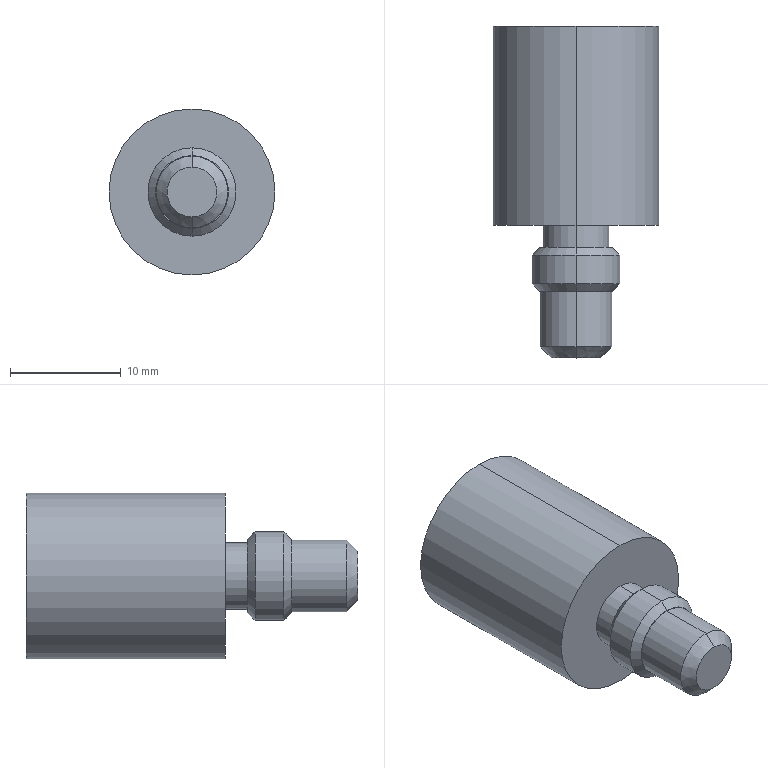Part | STEP file | X77-09313 | 1 solid | 25 faces | box 15 x 30 x 15 mm | volume 3215 mm3 | cone 10 | cylinder 10 | plane 5 | commonest cylinder face diameters 6.5 x4 6 x2 8 x2 15 x2
STEP:
#1=CARTESIAN_POINT('',(0.,28.,-3.25));
#2=VERTEX_POINT('',#1);
#3=CARTESIAN_POINT('',(0.,28.,3.25));
#4=VERTEX_POINT('',#3);
#5=CARTESIAN_POINT('',(0.,28.,0.));
#6=DIRECTION('',(0.,1.,0.));
#7=DIRECTION('',(0.,0.,-1.));
#8=AXIS2_PLACEMENT_3D('',#5,#6,#7);
#9=CIRCLE('',#8,3.25);
#10=EDGE_CURVE('',#2,#4,#9,.T.);
#11=ORIENTED_EDGE('',*,*,#10,.F.);
#12=CARTESIAN_POINT('',(0.,30.,-5.25));
#13=VERTEX_POINT('',#12);
#14=CARTESIAN_POINT('',(0.,30.,-5.25));
#15=DIRECTION('',(0.,0.7071,-0.7071));
#16=VECTOR('',#15,1000.);
#17=LINE('',#14,#16);
#18=EDGE_CURVE('',#2,#13,#17,.T.);
#19=ORIENTED_EDGE('',*,*,#18,.T.);
#20=CARTESIAN_POINT('',(0.,30.,5.25));
#21=VERTEX_POINT('',#20);
#22=CARTESIAN_POINT('',(0.,30.,0.));
#23=DIRECTION('',(0.,-1.,0.));
#24=DIRECTION('',(0.,0.,-1.));
#25=AXIS2_PLACEMENT_3D('',#22,#23,#24);
#26=CIRCLE('',#25,5.25);
#27=EDGE_CURVE('',#21,#13,#26,.T.);
#28=ORIENTED_EDGE('',*,*,#27,.F.);
#29=CARTESIAN_POINT('',(0.,30.,5.25));
#30=DIRECTION('',(0.,0.7071,0.7071));
#31=VECTOR('',#30,1000.);
#32=LINE('',#29,#31);
#33=EDGE_CURVE('',#4,#21,#32,.T.);
#34=ORIENTED_EDGE('',*,*,#33,.F.);
#35=EDGE_LOOP('',(#11,#19,#28,#34));
#36=FACE_OUTER_BOUND('',#35,.T.);
#37=CARTESIAN_POINT('',(0.,30.,0.));
#38=DIRECTION('',(0.,1.,0.));
#39=DIRECTION('',(0.,0.,1.));
#40=AXIS2_PLACEMENT_3D('',#37,#38,#39);
#41=CONICAL_SURFACE('',#40,5.25,0.7854);
#42=ADVANCED_FACE('',(#36),#41,.F.);
#43=CARTESIAN_POINT('',(0.,0.,-2.25));
#44=VERTEX_POINT('',#43);
#45=CARTESIAN_POINT('',(0.,0.,2.25));
#46=VERTEX_POINT('',#45);
#47=CARTESIAN_POINT('',(0.,0.,0.));
#48=DIRECTION('',(0.,-1.,0.));
#49=DIRECTION('',(0.,0.,-1.));
#50=AXIS2_PLACEMENT_3D('',#47,#48,#49);
#51=CIRCLE('',#50,2.25);
#52=EDGE_CURVE('',#44,#46,#51,.T.);
#53=ORIENTED_EDGE('',*,*,#52,.F.);
#54=CARTESIAN_POINT('',(0.,1.,-3.25));
#55=VERTEX_POINT('',#54);
#56=CARTESIAN_POINT('',(0.,1.,-3.25));
#57=DIRECTION('',(0.,0.7071,-0.7071));
#58=VECTOR('',#57,1000.);
#59=LINE('',#56,#58);
#60=EDGE_CURVE('',#44,#55,#59,.T.);
#61=ORIENTED_EDGE('',*,*,#60,.T.);
#62=CARTESIAN_POINT('',(0.,1.,3.25));
#63=VERTEX_POINT('',#62);
#64=CARTESIAN_POINT('',(0.,1.,0.));
#65=DIRECTION('',(0.,-1.,0.));
#66=DIRECTION('',(0.,0.,-1.));
#67=AXIS2_PLACEMENT_3D('',#64,#65,#66);
#68=CIRCLE('',#67,3.25);
#69=EDGE_CURVE('',#55,#63,#68,.T.);
#70=ORIENTED_EDGE('',*,*,#69,.T.);
#71=CARTESIAN_POINT('',(0.,1.,3.25));
#72=DIRECTION('',(0.,0.7071,0.7071));
#73=VECTOR('',#72,1000.);
#74=LINE('',#71,#73);
#75=EDGE_CURVE('',#46,#63,#74,.T.);
#76=ORIENTED_EDGE('',*,*,#75,.F.);
#77=EDGE_LOOP('',(#53,#61,#70,#76));
#78=FACE_OUTER_BOUND('',#77,.T.);
#79=CARTESIAN_POINT('',(0.,1.,0.));
#80=DIRECTION('',(0.,1.,0.));
#81=DIRECTION('',(0.,0.,1.));
#82=AXIS2_PLACEMENT_3D('',#79,#80,#81);
#83=CONICAL_SURFACE('',#82,3.25,0.7854);
#84=ADVANCED_FACE('',(#78),#83,.T.);
#85=CARTESIAN_POINT('',(0.,6.,-3.25));
#86=VERTEX_POINT('',#85);
#87=CARTESIAN_POINT('',(0.,6.,3.25));
#88=VERTEX_POINT('',#87);
#89=CARTESIAN_POINT('',(0.,6.,0.));
#90=DIRECTION('',(0.,-1.,0.));
#91=DIRECTION('',(0.,0.,-1.));
#92=AXIS2_PLACEMENT_3D('',#89,#90,#91);
#93=CIRCLE('',#92,3.25);
#94=EDGE_CURVE('',#86,#88,#93,.T.);
#95=ORIENTED_EDGE('',*,*,#94,.T.);
#96=CARTESIAN_POINT('',(0.,0.,3.25));
#97=DIRECTION('',(0.,-1.,0.));
#98=VECTOR('',#97,1000.);
#99=LINE('',#96,#98);
#100=EDGE_CURVE('',#88,#63,#99,.T.);
#101=ORIENTED_EDGE('',*,*,#100,.T.);
#102=ORIENTED_EDGE('',*,*,#69,.F.);
#103=CARTESIAN_POINT('',(0.,0.,-3.25));
#104=DIRECTION('',(0.,-1.,0.));
#105=VECTOR('',#104,1000.);
#106=LINE('',#103,#105);
#107=EDGE_CURVE('',#86,#55,#106,.T.);
#108=ORIENTED_EDGE('',*,*,#107,.F.);
#109=EDGE_LOOP('',(#95,#101,#102,#108));
#110=FACE_OUTER_BOUND('',#109,.T.);
#111=CARTESIAN_POINT('',(0.,0.,0.));
#112=DIRECTION('',(0.,-1.,0.));
#113=DIRECTION('',(0.,0.,-1.));
#114=AXIS2_PLACEMENT_3D('',#111,#112,#113);
#115=CYLINDRICAL_SURFACE('',#114,3.25);
#116=ADVANCED_FACE('',(#110),#115,.T.);
#117=CARTESIAN_POINT('',(0.,6.,-3.3));
#118=VERTEX_POINT('',#117);
#119=CARTESIAN_POINT('',(0.,6.,3.3));
#120=VERTEX_POINT('',#119);
#121=CARTESIAN_POINT('',(0.,6.,0.));
#122=DIRECTION('',(0.,-1.,0.));
#123=DIRECTION('',(0.,0.,-1.));
#124=AXIS2_PLACEMENT_3D('',#121,#122,#123);
#125=CIRCLE('',#124,3.3);
#126=EDGE_CURVE('',#118,#120,#125,.T.);
#127=ORIENTED_EDGE('',*,*,#126,.F.);
#128=CARTESIAN_POINT('',(0.,6.7,-4.));
#129=VERTEX_POINT('',#128);
#130=CARTESIAN_POINT('',(0.,6.7,-4.));
#131=DIRECTION('',(0.,0.7071,-0.7071));
#132=VECTOR('',#131,1000.);
#133=LINE('',#130,#132);
#134=EDGE_CURVE('',#118,#129,#133,.T.);
#135=ORIENTED_EDGE('',*,*,#134,.T.);
#136=CARTESIAN_POINT('',(0.,6.7,4.));
#137=VERTEX_POINT('',#136);
#138=CARTESIAN_POINT('',(0.,6.7,0.));
#139=DIRECTION('',(0.,-1.,0.));
#140=DIRECTION('',(0.,0.,-1.));
#141=AXIS2_PLACEMENT_3D('',#138,#139,#140);
#142=CIRCLE('',#141,4.);
#143=EDGE_CURVE('',#129,#137,#142,.T.);
#144=ORIENTED_EDGE('',*,*,#143,.T.);
#145=CARTESIAN_POINT('',(0.,6.7,4.));
#146=DIRECTION('',(0.,0.7071,0.7071));
#147=VECTOR('',#146,1000.);
#148=LINE('',#145,#147);
#149=EDGE_CURVE('',#120,#137,#148,.T.);
#150=ORIENTED_EDGE('',*,*,#149,.F.);
#151=EDGE_LOOP('',(#127,#135,#144,#150));
#152=FACE_OUTER_BOUND('',#151,.T.);
#153=CARTESIAN_POINT('',(0.,6.7,0.));
#154=DIRECTION('',(0.,1.,0.));
#155=DIRECTION('',(0.,0.,1.));
#156=AXIS2_PLACEMENT_3D('',#153,#154,#155);
#157=CONICAL_SURFACE('',#156,4.,0.7854);
#158=ADVANCED_FACE('',(#152),#157,.T.);
#159=CARTESIAN_POINT('',(0.,9.3,-4.));
#160=VERTEX_POINT('',#159);
#161=CARTESIAN_POINT('',(0.,9.3,4.));
#162=VERTEX_POINT('',#161);
#163=CARTESIAN_POINT('',(0.,9.3,0.));
#164=DIRECTION('',(0.,-1.,0.));
#165=DIRECTION('',(0.,0.,-1.));
#166=AXIS2_PLACEMENT_3D('',#163,#164,#165);
#167=CIRCLE('',#166,4.);
#168=EDGE_CURVE('',#160,#162,#167,.T.);
#169=ORIENTED_EDGE('',*,*,#168,.T.);
#170=CARTESIAN_POINT('',(0.,0.,4.));
#171=DIRECTION('',(0.,-1.,0.));
#172=VECTOR('',#171,1000.);
#173=LINE('',#170,#172);
#174=EDGE_CURVE('',#162,#137,#173,.T.);
#175=ORIENTED_EDGE('',*,*,#174,.T.);
#176=ORIENTED_EDGE('',*,*,#143,.F.);
#177=CARTESIAN_POINT('',(0.,0.,-4.));
#178=DIRECTION('',(0.,-1.,0.));
#179=VECTOR('',#178,1000.);
#180=LINE('',#177,#179);
#181=EDGE_CURVE('',#160,#129,#180,.T.);
#182=ORIENTED_EDGE('',*,*,#181,.F.);
#183=EDGE_LOOP('',(#169,#175,#176,#182));
#184=FACE_OUTER_BOUND('',#183,.T.);
#185=CARTESIAN_POINT('',(0.,0.,0.));
#186=DIRECTION('',(0.,-1.,0.));
#187=DIRECTION('',(0.,0.,-1.));
#188=AXIS2_PLACEMENT_3D('',#185,#186,#187);
#189=CYLINDRICAL_SURFACE('',#188,4.);
#190=ADVANCED_FACE('',(#184),#189,.T.);
#191=CARTESIAN_POINT('',(0.,10.,-3.3));
#192=VERTEX_POINT('',#191);
#193=CARTESIAN_POINT('',(0.,10.,3.3));
#194=VERTEX_POINT('',#193);
#195=CARTESIAN_POINT('',(0.,10.,0.));
#196=DIRECTION('',(0.,-1.,0.));
#197=DIRECTION('',(0.,0.,-1.));
#198=AXIS2_PLACEMENT_3D('',#195,#196,#197);
#199=CIRCLE('',#198,3.3);
#200=EDGE_CURVE('',#192,#194,#199,.T.);
#201=ORIENTED_EDGE('',*,*,#200,.T.);
#202=CARTESIAN_POINT('',(0.,10.,3.3));
#203=DIRECTION('',(0.,-0.7071,0.7071));
#204=VECTOR('',#203,1000.);
#205=LINE('',#202,#204);
#206=EDGE_CURVE('',#194,#162,#205,.T.);
#207=ORIENTED_EDGE('',*,*,#206,.T.);
#208=ORIENTED_EDGE('',*,*,#168,.F.);
#209=CARTESIAN_POINT('',(0.,10.,-3.3));
#210=DIRECTION('',(0.,-0.7071,-0.7071));
#211=VECTOR('',#210,1000.);
#212=LINE('',#209,#211);
#213=EDGE_CURVE('',#192,#160,#212,.T.);
#214=ORIENTED_EDGE('',*,*,#213,.F.);
#215=EDGE_LOOP('',(#201,#207,#208,#214));
#216=FACE_OUTER_BOUND('',#215,.T.);
#217=CARTESIAN_POINT('',(0.,10.,0.));
#218=DIRECTION('',(0.,-1.,0.));
#219=DIRECTION('',(0.,0.,-1.));
#220=AXIS2_PLACEMENT_3D('',#217,#218,#219);
#221=CONICAL_SURFACE('',#220,3.3,0.7854);
#222=ADVANCED_FACE('',(#216),#221,.T.);
#223=CARTESIAN_POINT('',(0.,12.,-3.));
#224=VERTEX_POINT('',#223);
#225=CARTESIAN_POINT('',(0.,12.,3.));
#226=VERTEX_POINT('',#225);
#227=CARTESIAN_POINT('',(0.,12.,0.));
#228=DIRECTION('',(0.,-1.,0.));
#229=DIRECTION('',(0.,0.,-1.));
#230=AXIS2_PLACEMENT_3D('',#227,#228,#229);
#231=CIRCLE('',#230,3.);
#232=EDGE_CURVE('',#224,#226,#231,.T.);
#233=ORIENTED_EDGE('',*,*,#232,.T.);
#234=CARTESIAN_POINT('',(0.,10.,3.));
#235=VERTEX_POINT('',#234);
#236=CARTESIAN_POINT('',(0.,0.,3.));
#237=DIRECTION('',(0.,-1.,0.));
#238=VECTOR('',#237,1000.);
#239=LINE('',#236,#238);
#240=EDGE_CURVE('',#226,#235,#239,.T.);
#241=ORIENTED_EDGE('',*,*,#240,.T.);
#242=CARTESIAN_POINT('',(0.,10.,-3.));
#243=VERTEX_POINT('',#242);
#244=CARTESIAN_POINT('',(0.,10.,0.));
#245=DIRECTION('',(0.,-1.,0.));
#246=DIRECTION('',(0.,0.,-1.));
#247=AXIS2_PLACEMENT_3D('',#244,#245,#246);
#248=CIRCLE('',#247,3.);
#249=EDGE_CURVE('',#243,#235,#248,.T.);
#250=ORIENTED_EDGE('',*,*,#249,.F.);
#251=CARTESIAN_POINT('',(0.,0.,-3.));
#252=DIRECTION('',(0.,-1.,0.));
#253=VECTOR('',#252,1000.);
#254=LINE('',#251,#253);
#255=EDGE_CURVE('',#224,#243,#254,.T.);
#256=ORIENTED_EDGE('',*,*,#255,.F.);
#257=EDGE_LOOP('',(#233,#241,#250,#256));
#258=FACE_OUTER_BOUND('',#257,.T.);
#259=CARTESIAN_POINT('',(0.,0.,0.));
#260=DIRECTION('',(0.,-1.,0.));
#261=DIRECTION('',(0.,0.,-1.));
#262=AXIS2_PLACEMENT_3D('',#259,#260,#261);
#263=CYLINDRICAL_SURFACE('',#262,3.);
#264=ADVANCED_FACE('',(#258),#263,.T.);
#265=CARTESIAN_POINT('',(0.,30.,-7.5));
#266=VERTEX_POINT('',#265);
#267=CARTESIAN_POINT('',(0.,30.,7.5));
#268=VERTEX_POINT('',#267);
#269=CARTESIAN_POINT('',(0.,30.,0.));
#270=DIRECTION('',(0.,-1.,0.));
#271=DIRECTION('',(0.,0.,-1.));
#272=AXIS2_PLACEMENT_3D('',#269,#270,#271);
#273=CIRCLE('',#272,7.5);
#274=EDGE_CURVE('',#266,#268,#273,.T.);
#275=ORIENTED_EDGE('',*,*,#274,.T.);
#276=CARTESIAN_POINT('',(0.,12.,7.5));
#277=VERTEX_POINT('',#276);
#278=CARTESIAN_POINT('',(0.,0.,7.5));
#279=DIRECTION('',(0.,-1.,0.));
#280=VECTOR('',#279,1000.);
#281=LINE('',#278,#280);
#282=EDGE_CURVE('',#268,#277,#281,.T.);
#283=ORIENTED_EDGE('',*,*,#282,.T.);
#284=CARTESIAN_POINT('',(0.,12.,-7.5));
#285=VERTEX_POINT('',#284);
#286=CARTESIAN_POINT('',(0.,12.,0.));
#287=DIRECTION('',(0.,-1.,0.));
#288=DIRECTION('',(0.,0.,-1.));
#289=AXIS2_PLACEMENT_3D('',#286,#287,#288);
#290=CIRCLE('',#289,7.5);
#291=EDGE_CURVE('',#285,#277,#290,.T.);
#292=ORIENTED_EDGE('',*,*,#291,.F.);
#293=CARTESIAN_POINT('',(0.,0.,-7.5));
#294=DIRECTION('',(0.,-1.,0.));
#295=VECTOR('',#294,1000.);
#296=LINE('',#293,#295);
#297=EDGE_CURVE('',#266,#285,#296,.T.);
#298=ORIENTED_EDGE('',*,*,#297,.F.);
#299=EDGE_LOOP('',(#275,#283,#292,#298));
#300=FACE_OUTER_BOUND('',#299,.T.);
#301=CARTESIAN_POINT('',(0.,0.,0.));
#302=DIRECTION('',(0.,-1.,0.));
#303=DIRECTION('',(0.,0.,-1.));
#304=AXIS2_PLACEMENT_3D('',#301,#302,#303);
#305=CYLINDRICAL_SURFACE('',#304,7.5);
#306=ADVANCED_FACE('',(#300),#305,.T.);
#307=ORIENTED_EDGE('',*,*,#10,.T.);
#308=CARTESIAN_POINT('',(0.,20.,3.25));
#309=VERTEX_POINT('',#308);
#310=CARTESIAN_POINT('',(0.,0.,3.25));
#311=DIRECTION('',(0.,-1.,0.));
#312=VECTOR('',#311,1000.);
#313=LINE('',#310,#312);
#314=EDGE_CURVE('',#4,#309,#313,.T.);
#315=ORIENTED_EDGE('',*,*,#314,.T.);
#316=CARTESIAN_POINT('',(0.,20.,-3.25));
#317=VERTEX_POINT('',#316);
#318=CARTESIAN_POINT('',(0.,20.,0.));
#319=DIRECTION('',(0.,-1.,0.));
#320=DIRECTION('',(0.,0.,-1.));
#321=AXIS2_PLACEMENT_3D('',#318,#319,#320);
#322=CIRCLE('',#321,3.25);
#323=EDGE_CURVE('',#309,#317,#322,.T.);
#324=ORIENTED_EDGE('',*,*,#323,.T.);
#325=CARTESIAN_POINT('',(0.,0.,-3.25));
#326=DIRECTION('',(0.,-1.,0.));
#327=VECTOR('',#326,1000.);
#328=LINE('',#325,#327);
#329=EDGE_CURVE('',#2,#317,#328,.T.);
#330=ORIENTED_EDGE('',*,*,#329,.F.);
#331=EDGE_LOOP('',(#307,#315,#324,#330));
#332=FACE_OUTER_BOUND('',#331,.T.);
#333=CARTESIAN_POINT('',(0.,0.,0.));
#334=DIRECTION('',(0.,-1.,0.));
#335=DIRECTION('',(0.,0.,-1.));
#336=AXIS2_PLACEMENT_3D('',#333,#334,#335);
#337=CYLINDRICAL_SURFACE('',#336,3.25);
#338=ADVANCED_FACE('',(#332),#337,.F.);
#339=CARTESIAN_POINT('',(0.,18.124,0.));
#340=VERTEX_POINT('',#339);
#341=CARTESIAN_POINT('',(0.,18.124,0.));
#342=DIRECTION('',(0.,0.5,0.866));
#343=VECTOR('',#342,1000.);
#344=LINE('',#341,#343);
#345=EDGE_CURVE('',#340,#309,#344,.T.);
#346=ORIENTED_EDGE('',*,*,#345,.F.);
#347=CARTESIAN_POINT('',(0.,18.124,0.));
#348=DIRECTION('',(0.,0.5,-0.866));
#349=VECTOR('',#348,1000.);
#350=LINE('',#347,#349);
#351=EDGE_CURVE('',#340,#317,#350,.T.);
#352=ORIENTED_EDGE('',*,*,#351,.T.);
#353=ORIENTED_EDGE('',*,*,#323,.F.);
#354=EDGE_LOOP('',(#346,#352,#353));
#355=FACE_OUTER_BOUND('',#354,.T.);
#356=CARTESIAN_POINT('',(0.,1018.124,0.));
#357=DIRECTION('',(0.,1.,0.));
#358=DIRECTION('',(0.,0.,1.));
#359=AXIS2_PLACEMENT_3D('',#356,#357,#358);
#360=CONICAL_SURFACE('',#359,1732.051,1.047);
#361=ADVANCED_FACE('',(#355),#360,.F.);
#362=ORIENTED_EDGE('',*,*,#351,.F.);
#363=ORIENTED_EDGE('',*,*,#345,.T.);
#364=CARTESIAN_POINT('',(0.,20.,0.));
#365=DIRECTION('',(0.,-1.,0.));
#366=DIRECTION('',(0.,0.,-1.));
#367=AXIS2_PLACEMENT_3D('',#364,#365,#366);
#368=CIRCLE('',#367,3.25);
#369=EDGE_CURVE('',#317,#309,#368,.T.);
#370=ORIENTED_EDGE('',*,*,#369,.F.);
#371=EDGE_LOOP('',(#362,#363,#370));
#372=FACE_OUTER_BOUND('',#371,.T.);
#373=CARTESIAN_POINT('',(0.,1018.124,0.));
#374=DIRECTION('',(0.,1.,0.));
#375=DIRECTION('',(0.,0.,1.));
#376=AXIS2_PLACEMENT_3D('',#373,#374,#375);
#377=CONICAL_SURFACE('',#376,1732.051,1.047);
#378=ADVANCED_FACE('',(#372),#377,.F.);
#379=ORIENTED_EDGE('',*,*,#314,.F.);
#380=CARTESIAN_POINT('',(0.,28.,0.));
#381=DIRECTION('',(0.,1.,0.));
#382=DIRECTION('',(0.,0.,-1.));
#383=AXIS2_PLACEMENT_3D('',#380,#381,#382);
#384=CIRCLE('',#383,3.25);
#385=EDGE_CURVE('',#4,#2,#384,.T.);
#386=ORIENTED_EDGE('',*,*,#385,.T.);
#387=ORIENTED_EDGE('',*,*,#329,.T.);
#388=ORIENTED_EDGE('',*,*,#369,.T.);
#389=EDGE_LOOP('',(#379,#386,#387,#388));
#390=FACE_OUTER_BOUND('',#389,.T.);
#391=CARTESIAN_POINT('',(0.,0.,0.));
#392=DIRECTION('',(0.,-1.,0.));
#393=DIRECTION('',(0.,0.,-1.));
#394=AXIS2_PLACEMENT_3D('',#391,#392,#393);
#395=CYLINDRICAL_SURFACE('',#394,3.25);
#396=ADVANCED_FACE('',(#390),#395,.F.);
#397=ORIENTED_EDGE('',*,*,#27,.T.);
#398=CARTESIAN_POINT('',(0.,30.,0.));
#399=DIRECTION('',(0.,-1.,0.));
#400=DIRECTION('',(0.,0.,-1.));
#401=AXIS2_PLACEMENT_3D('',#398,#399,#400);
#402=CIRCLE('',#401,5.25);
#403=EDGE_CURVE('',#13,#21,#402,.T.);
#404=ORIENTED_EDGE('',*,*,#403,.T.);
#405=EDGE_LOOP('',(#397,#404));
#406=FACE_BOUND('',#405,.T.);
#407=ORIENTED_EDGE('',*,*,#274,.F.);
#408=CARTESIAN_POINT('',(0.,30.,0.));
#409=DIRECTION('',(0.,-1.,0.));
#410=DIRECTION('',(0.,0.,-1.));
#411=AXIS2_PLACEMENT_3D('',#408,#409,#410);
#412=CIRCLE('',#411,7.5);
#413=EDGE_CURVE('',#268,#266,#412,.T.);
#414=ORIENTED_EDGE('',*,*,#413,.F.);
#415=EDGE_LOOP('',(#407,#414));
#416=FACE_OUTER_BOUND('',#415,.T.);
#417=CARTESIAN_POINT('',(-3.25,30.,0.));
#418=DIRECTION('',(0.,-1.,0.));
#419=DIRECTION('',(0.,0.,-1.));
#420=AXIS2_PLACEMENT_3D('',#417,#418,#419);
#421=PLANE('',#420);
#422=ADVANCED_FACE('',(#406,#416),#421,.F.);
#423=ORIENTED_EDGE('',*,*,#282,.F.);
#424=ORIENTED_EDGE('',*,*,#413,.T.);
#425=ORIENTED_EDGE('',*,*,#297,.T.);
#426=CARTESIAN_POINT('',(0.,12.,0.));
#427=DIRECTION('',(0.,-1.,0.));
#428=DIRECTION('',(0.,0.,-1.));
#429=AXIS2_PLACEMENT_3D('',#426,#427,#428);
#430=CIRCLE('',#429,7.5);
#431=EDGE_CURVE('',#277,#285,#430,.T.);
#432=ORIENTED_EDGE('',*,*,#431,.F.);
#433=EDGE_LOOP('',(#423,#424,#425,#432));
#434=FACE_OUTER_BOUND('',#433,.T.);
#435=CARTESIAN_POINT('',(0.,0.,0.));
#436=DIRECTION('',(0.,-1.,0.));
#437=DIRECTION('',(0.,0.,-1.));
#438=AXIS2_PLACEMENT_3D('',#435,#436,#437);
#439=CYLINDRICAL_SURFACE('',#438,7.5);
#440=ADVANCED_FACE('',(#434),#439,.T.);
#441=ORIENTED_EDGE('',*,*,#232,.F.);
#442=CARTESIAN_POINT('',(0.,12.,0.));
#443=DIRECTION('',(0.,-1.,0.));
#444=DIRECTION('',(0.,0.,-1.));
#445=AXIS2_PLACEMENT_3D('',#442,#443,#444);
#446=CIRCLE('',#445,3.);
#447=EDGE_CURVE('',#226,#224,#446,.T.);
#448=ORIENTED_EDGE('',*,*,#447,.F.);
#449=EDGE_LOOP('',(#441,#448));
#450=FACE_BOUND('',#449,.T.);
#451=ORIENTED_EDGE('',*,*,#291,.T.);
#452=ORIENTED_EDGE('',*,*,#431,.T.);
#453=EDGE_LOOP('',(#451,#452));
#454=FACE_OUTER_BOUND('',#453,.T.);
#455=CARTESIAN_POINT('',(-4.,12.,0.));
#456=DIRECTION('',(0.,1.,0.));
#457=DIRECTION('',(0.,0.,1.));
#458=AXIS2_PLACEMENT_3D('',#455,#456,#457);
#459=PLANE('',#458);
#460=ADVANCED_FACE('',(#450,#454),#459,.F.);
#461=ORIENTED_EDGE('',*,*,#240,.F.);
#462=ORIENTED_EDGE('',*,*,#447,.T.);
#463=ORIENTED_EDGE('',*,*,#255,.T.);
#464=CARTESIAN_POINT('',(0.,10.,0.));
#465=DIRECTION('',(0.,-1.,0.));
#466=DIRECTION('',(0.,0.,-1.));
#467=AXIS2_PLACEMENT_3D('',#464,#465,#466);
#468=CIRCLE('',#467,3.);
#469=EDGE_CURVE('',#235,#243,#468,.T.);
#470=ORIENTED_EDGE('',*,*,#469,.F.);
#471=EDGE_LOOP('',(#461,#462,#463,#470));
#472=FACE_OUTER_BOUND('',#471,.T.);
#473=CARTESIAN_POINT('',(0.,0.,0.));
#474=DIRECTION('',(0.,-1.,0.));
#475=DIRECTION('',(0.,0.,-1.));
#476=AXIS2_PLACEMENT_3D('',#473,#474,#475);
#477=CYLINDRICAL_SURFACE('',#476,3.);
#478=ADVANCED_FACE('',(#472),#477,.T.);
#479=ORIENTED_EDGE('',*,*,#200,.F.);
#480=CARTESIAN_POINT('',(0.,10.,0.));
#481=DIRECTION('',(0.,-1.,0.));
#482=DIRECTION('',(0.,0.,-1.));
#483=AXIS2_PLACEMENT_3D('',#480,#481,#482);
#484=CIRCLE('',#483,3.3);
#485=EDGE_CURVE('',#194,#192,#484,.T.);
#486=ORIENTED_EDGE('',*,*,#485,.F.);
#487=EDGE_LOOP('',(#479,#486));
#488=FACE_OUTER_BOUND('',#487,.T.);
#489=ORIENTED_EDGE('',*,*,#249,.T.);
#490=ORIENTED_EDGE('',*,*,#469,.T.);
#491=EDGE_LOOP('',(#489,#490));
#492=FACE_BOUND('',#491,.T.);
#493=CARTESIAN_POINT('',(-3.3,10.,0.));
#494=DIRECTION('',(0.,-1.,0.));
#495=DIRECTION('',(0.,0.,-1.));
#496=AXIS2_PLACEMENT_3D('',#493,#494,#495);
#497=PLANE('',#496);
#498=ADVANCED_FACE('',(#488,#492),#497,.F.);
#499=ORIENTED_EDGE('',*,*,#206,.F.);
#500=ORIENTED_EDGE('',*,*,#485,.T.);
#501=ORIENTED_EDGE('',*,*,#213,.T.);
#502=CARTESIAN_POINT('',(0.,9.3,0.));
#503=DIRECTION('',(0.,-1.,0.));
#504=DIRECTION('',(0.,0.,-1.));
#505=AXIS2_PLACEMENT_3D('',#502,#503,#504);
#506=CIRCLE('',#505,4.);
#507=EDGE_CURVE('',#162,#160,#506,.T.);
#508=ORIENTED_EDGE('',*,*,#507,.F.);
#509=EDGE_LOOP('',(#499,#500,#501,#508));
#510=FACE_OUTER_BOUND('',#509,.T.);
#511=CARTESIAN_POINT('',(0.,10.,0.));
#512=DIRECTION('',(0.,-1.,0.));
#513=DIRECTION('',(0.,0.,-1.));
#514=AXIS2_PLACEMENT_3D('',#511,#512,#513);
#515=CONICAL_SURFACE('',#514,3.3,0.7854);
#516=ADVANCED_FACE('',(#510),#515,.T.);
#517=ORIENTED_EDGE('',*,*,#174,.F.);
#518=ORIENTED_EDGE('',*,*,#507,.T.);
#519=ORIENTED_EDGE('',*,*,#181,.T.);
#520=CARTESIAN_POINT('',(0.,6.7,0.));
#521=DIRECTION('',(0.,-1.,0.));
#522=DIRECTION('',(0.,0.,-1.));
#523=AXIS2_PLACEMENT_3D('',#520,#521,#522);
#524=CIRCLE('',#523,4.);
#525=EDGE_CURVE('',#137,#129,#524,.T.);
#526=ORIENTED_EDGE('',*,*,#525,.F.);
#527=EDGE_LOOP('',(#517,#518,#519,#526));
#528=FACE_OUTER_BOUND('',#527,.T.);
#529=CARTESIAN_POINT('',(0.,0.,0.));
#530=DIRECTION('',(0.,-1.,0.));
#531=DIRECTION('',(0.,0.,-1.));
#532=AXIS2_PLACEMENT_3D('',#529,#530,#531);
#533=CYLINDRICAL_SURFACE('',#532,4.);
#534=ADVANCED_FACE('',(#528),#533,.T.);
#535=ORIENTED_EDGE('',*,*,#134,.F.);
#536=CARTESIAN_POINT('',(0.,6.,0.));
#537=DIRECTION('',(0.,-1.,0.));
#538=DIRECTION('',(0.,0.,-1.));
#539=AXIS2_PLACEMENT_3D('',#536,#537,#538);
#540=CIRCLE('',#539,3.3);
#541=EDGE_CURVE('',#120,#118,#540,.T.);
#542=ORIENTED_EDGE('',*,*,#541,.F.);
#543=ORIENTED_EDGE('',*,*,#149,.T.);
#544=ORIENTED_EDGE('',*,*,#525,.T.);
#545=EDGE_LOOP('',(#535,#542,#543,#544));
#546=FACE_OUTER_BOUND('',#545,.T.);
#547=CARTESIAN_POINT('',(0.,6.7,0.));
#548=DIRECTION('',(0.,1.,0.));
#549=DIRECTION('',(0.,0.,1.));
#550=AXIS2_PLACEMENT_3D('',#547,#548,#549);
#551=CONICAL_SURFACE('',#550,4.,0.7854);
#552=ADVANCED_FACE('',(#546),#551,.T.);
#553=ORIENTED_EDGE('',*,*,#94,.F.);
#554=CARTESIAN_POINT('',(0.,6.,0.));
#555=DIRECTION('',(0.,-1.,0.));
#556=DIRECTION('',(0.,0.,-1.));
#557=AXIS2_PLACEMENT_3D('',#554,#555,#556);
#558=CIRCLE('',#557,3.25);
#559=EDGE_CURVE('',#88,#86,#558,.T.);
#560=ORIENTED_EDGE('',*,*,#559,.F.);
#561=EDGE_LOOP('',(#553,#560));
#562=FACE_BOUND('',#561,.T.);
#563=ORIENTED_EDGE('',*,*,#541,.T.);
#564=ORIENTED_EDGE('',*,*,#126,.T.);
#565=EDGE_LOOP('',(#563,#564));
#566=FACE_OUTER_BOUND('',#565,.T.);
#567=CARTESIAN_POINT('',(-3.25,6.,0.));
#568=DIRECTION('',(0.,1.,0.));
#569=DIRECTION('',(0.,0.,1.));
#570=AXIS2_PLACEMENT_3D('',#567,#568,#569);
#571=PLANE('',#570);
#572=ADVANCED_FACE('',(#562,#566),#571,.F.);
#573=ORIENTED_EDGE('',*,*,#100,.F.);
#574=ORIENTED_EDGE('',*,*,#559,.T.);
#575=ORIENTED_EDGE('',*,*,#107,.T.);
#576=CARTESIAN_POINT('',(0.,1.,0.));
#577=DIRECTION('',(0.,-1.,0.));
#578=DIRECTION('',(0.,0.,-1.));
#579=AXIS2_PLACEMENT_3D('',#576,#577,#578);
#580=CIRCLE('',#579,3.25);
#581=EDGE_CURVE('',#63,#55,#580,.T.);
#582=ORIENTED_EDGE('',*,*,#581,.F.);
#583=EDGE_LOOP('',(#573,#574,#575,#582));
#584=FACE_OUTER_BOUND('',#583,.T.);
#585=CARTESIAN_POINT('',(0.,0.,0.));
#586=DIRECTION('',(0.,-1.,0.));
#587=DIRECTION('',(0.,0.,-1.));
#588=AXIS2_PLACEMENT_3D('',#585,#586,#587);
#589=CYLINDRICAL_SURFACE('',#588,3.25);
#590=ADVANCED_FACE('',(#584),#589,.T.);
#591=ORIENTED_EDGE('',*,*,#60,.F.);
#592=CARTESIAN_POINT('',(0.,0.,0.));
#593=DIRECTION('',(0.,-1.,0.));
#594=DIRECTION('',(0.,0.,-1.));
#595=AXIS2_PLACEMENT_3D('',#592,#593,#594);
#596=CIRCLE('',#595,2.25);
#597=EDGE_CURVE('',#46,#44,#596,.T.);
#598=ORIENTED_EDGE('',*,*,#597,.F.);
#599=ORIENTED_EDGE('',*,*,#75,.T.);
#600=ORIENTED_EDGE('',*,*,#581,.T.);
#601=EDGE_LOOP('',(#591,#598,#599,#600));
#602=FACE_OUTER_BOUND('',#601,.T.);
#603=CARTESIAN_POINT('',(0.,1.,0.));
#604=DIRECTION('',(0.,1.,0.));
#605=DIRECTION('',(0.,0.,1.));
#606=AXIS2_PLACEMENT_3D('',#603,#604,#605);
#607=CONICAL_SURFACE('',#606,3.25,0.7854);
#608=ADVANCED_FACE('',(#602),#607,.T.);
#609=ORIENTED_EDGE('',*,*,#597,.T.);
#610=ORIENTED_EDGE('',*,*,#52,.T.);
#611=EDGE_LOOP('',(#609,#610));
#612=FACE_OUTER_BOUND('',#611,.T.);
#613=CARTESIAN_POINT('',(-2.25,0.,0.));
#614=DIRECTION('',(0.,1.,0.));
#615=DIRECTION('',(0.,0.,1.));
#616=AXIS2_PLACEMENT_3D('',#613,#614,#615);
#617=PLANE('',#616);
#618=ADVANCED_FACE('',(#612),#617,.F.);
#619=ORIENTED_EDGE('',*,*,#18,.F.);
#620=ORIENTED_EDGE('',*,*,#385,.F.);
#621=ORIENTED_EDGE('',*,*,#33,.T.);
#622=ORIENTED_EDGE('',*,*,#403,.F.);
#623=EDGE_LOOP('',(#619,#620,#621,#622));
#624=FACE_OUTER_BOUND('',#623,.T.);
#625=CARTESIAN_POINT('',(0.,30.,0.));
#626=DIRECTION('',(0.,1.,0.));
#627=DIRECTION('',(0.,0.,1.));
#628=AXIS2_PLACEMENT_3D('',#625,#626,#627);
#629=CONICAL_SURFACE('',#628,5.25,0.7854);
#630=ADVANCED_FACE('',(#624),#629,.F.);
#631=CLOSED_SHELL('',(#42,#84,#116,#158,#190,#222,#264,#306,#338,#361,#378,#396,#422,#440,#460,#478,#498,#516,#534,#552,#572,#590,#608,#618,#630));
#632=MANIFOLD_SOLID_BREP('',#631);
#633=CARTESIAN_POINT('',(0.,0.,0.));
#634=DIRECTION('',(0.,0.,1.));
#635=DIRECTION('',(1.,0.,0.));
#636=AXIS2_PLACEMENT_3D('',#633,#634,#635);
#637=(LENGTH_UNIT()NAMED_UNIT(*)SI_UNIT(.MILLI.,.METRE.));
#638=UNCERTAINTY_MEASURE_WITH_UNIT(LENGTH_MEASURE(0.00001),#637,'','');
#639=(NAMED_UNIT(*)PLANE_ANGLE_UNIT()SI_UNIT($,.RADIAN.));
#640=(NAMED_UNIT(*)SI_UNIT($,.STERADIAN.)SOLID_ANGLE_UNIT());
#641=(GEOMETRIC_REPRESENTATION_CONTEXT(3)GLOBAL_UNCERTAINTY_ASSIGNED_CONTEXT((#638))GLOBAL_UNIT_ASSIGNED_CONTEXT((#637,#639,#640))REPRESENTATION_CONTEXT('',''));
#642=ADVANCED_BREP_SHAPE_REPRESENTATION('',(#632,#636),#641);